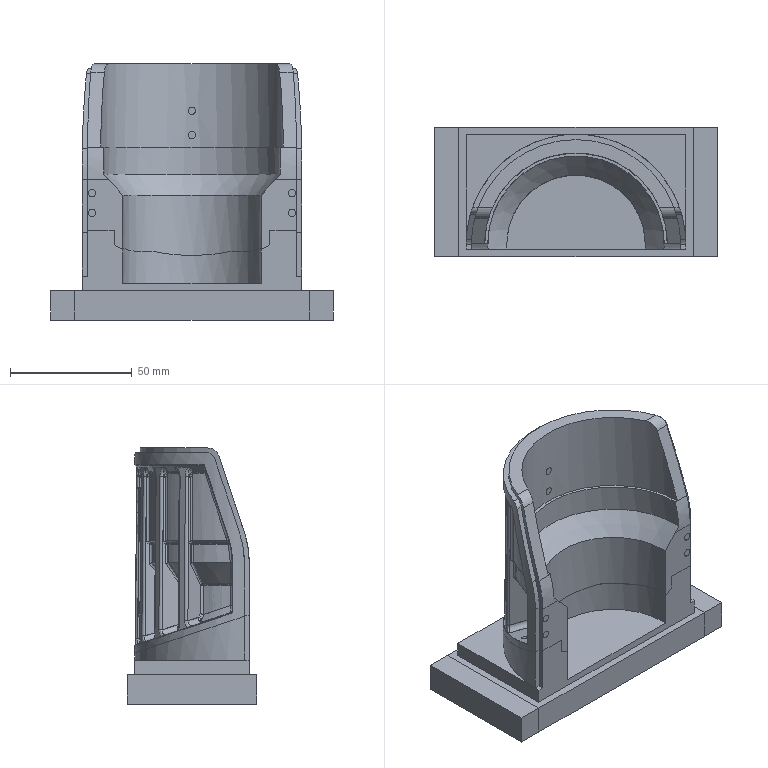CAM job | NX | 3-axis milling, 5-axis milling | part box 116 x 53 x 105 mm
Tools:
number,name,description,diameter,corner_radius,flute_length,length,flutes
16,J-D16,Milling Tool-5 Parameters,16.0,0.0,40.0,80.0,21
18,C-D10,Milling Tool-5 Parameters,10.0,0.0,30.0,45.0,21
14,C-D8,Milling Tool-5 Parameters,8.0,0.0,20.0,35.0,21
12,C-D4,Milling Tool-5 Parameters,4.0,0.0,10.0,25.0,21
6,C-D4R2,Milling Tool-5 Parameters,4.0,2.0,10.0,25.0,21
12,J-D4,Milling Tool-5 Parameters,4.0,0.0,10.0,25.0,21
10,J-D2,Milling Tool-5 Parameters,2.0,0.0,6.0,8.0,21
22,J-D10R0.5,Milling Tool-5 Parameters,10.0,0.5,30.0,55.0,21
21,J-D2R0.2,Milling Tool-5 Parameters,2.0,0.2,6.0,6.0,21
6,J-D4R2,Milling Tool-Ball Mill,4.0,2.0,10.0,25.0,2
8,J-D2R1,Milling Tool-Ball Mill,2.0,1.0,6.0,6.0,2
9,J-D1R0.5,Milling Tool-Ball Mill,1.0,0.5,3.0,3.0,2
7,J-D0.5R0.25,Milling Tool-5 Parameters,0.5,0.25,2.0,2.0,21
Operations:
program,operation,operation_type,tool,method,geometry_group,spindle_rpm,surface_speed,feed_per_tooth,feed_cut,feed_plunge,cut_length_mm,path_length_mm,cut_time_min,machine_time_min
A1,精飞平面,FaceMilling,C-D10,END_MILL_MACRO,WP-1,7000.0,829.0,0.1515,1500.0,100.0,797.45,877.25,0.5316,0.5396
A1,动态开粗,SurfaceContour,C-D10,END_MILL_MACRO,WP-1,7000.0,0.0,0.0,3500.0,100.0,59852.399,81581.703,12.618,14.791
A1,动态开粗_COPY,SurfaceContour,C-D10,END_MILL_MACRO,WP-1,7000.0,0.0,0.0,3500.0,100.0,64037.473,77543.878,13.518,14.868
A1,底壁-跟随,VolumeBased25DMillingOperation,C-D10,METHOD,WP-1,7000.0,87.0,0.2143,500.0,100.0,720.345,878.17,1.441,1.456
A1,底壁-跟随_COPY,VolumeBased25DMillingOperation,C-D10,METHOD,WP-1,7000.0,87.0,0.2143,500.0,100.0,224.0,381.776,0.448,0.4638
A1,剩余铣粗,CavityMilling,C-D10,METHOD,WP-1,7000.0,100.0,0.1178,3500.0,100.0,9658.396,19375.124,2.76,3.731
A1,剩余铣粗_COPY,CavityMilling,C-D10,METHOD,WP-1,7000.0,100.0,0.1178,3500.0,100.0,7296.167,14032.108,2.085,2.758
A1,精爬面,SurfaceContour,C-D10,METHOD,WP-1,7000.0,219.911,0.0102,1500.0,100.0,5400.471,10074.737,3.6,4.068
A2,剩余铣粗_1,CavityMilling,C-D4,METHOD,WP-1,7000.0,100.0,0.1178,3500.0,100.0,3566.135,5871.644,1.019,1.249
A2,剩余铣粗_1_COPY,CavityMilling,C-D4,METHOD,WP-1,7000.0,100.0,0.1178,3500.0,100.0,3352.533,5292.02,0.9579,1.152
A2,剩余铣粗_1_COPY_COPY,CavityMilling,C-D4,METHOD,WP-1,7000.0,100.0,0.1178,3500.0,100.0,3259.975,3977.24,0.9314,1.003
A2,剩余铣粗_1_COPY_COPY_COPY,CavityMilling,C-D4,METHOD,WP-1,7000.0,100.0,0.1178,3500.0,100.0,4154.568,4839.04,1.187,1.256
A2,剩余铣粗_1_COPY_COPY_COPY_COPY,CavityMilling,C-D4,METHOD,WP-1,7000.0,100.0,0.1178,3500.0,100.0,4601.008,5199.555,1.315,1.374
A2,剩余铣粗_1_COPY_COPY_COPY_COPY_COPY,CavityMilling,C-D4,METHOD,WP-1,7000.0,100.0,0.1178,3500.0,100.0,4824.636,5468.098,1.379,1.443
A2,剩余铣粗_1_COPY_COPY_COPY_COPY_COPY_COPY,CavityMilling,C-D4,METHOD,WP-1,7000.0,100.0,0.1178,3500.0,100.0,4042.646,4722.087,1.155,1.223
A2,剩余铣粗_1_COPY_COPY_COPY_COPY_COPY_COPY_COPY,CavityMilling,C-D4,METHOD,WP-1,7000.0,100.0,0.1178,3500.0,100.0,3298.926,4234.6,0.9426,1.036
A2,等高混合,ZLevelMilling,C-D4,METHOD,WP-1,8000.0,122.0,0.0044,2500.0,250.0,1422.571,1699.939,0.5983,0.6261
A2,五轴外形轮廓,SurfaceContour,C-D4,METHOD,WP-1,3500.0,0.0,0.0,600.0,100.0,442.58,1012.272,0.7376,0.7946
A2,五轴外形轮廓_INSTANCE,SurfaceContour,C-D4,METHOD,WP-1,3500.0,0.0,0.0,600.0,100.0,442.58,1012.272,0.7376,0.7946
A2,小孔开粗1,CylinderMilling,C-D4,METHOD,1-A,7000.0,0.0,0.0,600.0,100.0,271.272,447.005,0.4521,0.4697
A2,精大孔-1,PlanarMilling,C-D4,METHOD,1-A,7000.0,188.0,0.0063,200.0,250.0,42.382,208.58,0.2056,0.2223
A3,小孔开粗1_1,CylinderMilling,J-D2,METHOD,1-A,7000.0,0.0,0.0,600.0,100.0,321.786,497.146,0.5363,0.5538
A3,小孔开粗1_1_COPY,CylinderMilling,J-D2,METHOD,1-A,7000.0,0.0,0.0,600.0,100.0,1219.353,1665.353,2.032,2.077
A4,顶面-单刀,SurfaceContour,J-D16,METHOD,WP-1,4000.0,0.0,0.0,500.0,100.0,133.562,139.418,0.2671,0.2677
A4,底壁-跟随_1,VolumeBased25DMillingOperation,J-D16,METHOD,WP-1,4000.0,87.0,0.2143,500.0,100.0,563.041,721.065,1.126,1.142
A4,底壁-跟随_1_COPY,VolumeBased25DMillingOperation,J-D16,METHOD,WP-1,4000.0,87.0,0.2143,500.0,100.0,236.899,394.875,0.4738,0.4896
A4,底壁-跟随_1_COPY_COPY,VolumeBased25DMillingOperation,J-D16,METHOD,WP-1,4000.0,87.0,0.2143,500.0,100.0,150.899,265.899,0.3018,0.3133
A4,底壁-跟随_1_COPY_COPY_COPY,VolumeBased25DMillingOperation,J-D16,METHOD,WP-1,4000.0,87.0,0.2143,500.0,100.0,150.899,265.899,0.3018,0.3133
A5,精外形-1,PlanarMilling,J-D16,METHOD,WP-1,2000.0,100.531,0.0095,400.0,250.0,209.09,534.409,0.5414,0.5739
A5,精外形-1_COPY,PlanarMilling,J-D16,METHOD,WP-1,2000.0,100.531,0.0095,400.0,250.0,208.179,575.005,0.5391,0.5758
A5,精外形-1_COPY_COPY,PlanarMilling,J-D16,METHOD,WP-1,2000.0,100.531,0.0095,400.0,250.0,287.905,514.838,0.738,0.7607
A6,等高混合_1,ZLevelMilling,J-D10R0.5,METHOD,WP-1,8000.0,122.0,0.0044,2500.0,250.0,7195.714,7374.63,2.889,2.907
A7,精爬面_1,SurfaceContour,C-D4R2,METHOD,WP-1,9000.0,0.0,0.0,3500.0,100.0,1893.178,2136.544,0.5409,0.5652
A7,可变轴引导,SurfaceContour,C-D4R2,METHOD,WP-1,9000.0,0.0,0.0,3500.0,250.0,6901.077,6940.344,1.988,1.992
A7,可变轴引导_COPY,SurfaceContour,C-D4R2,METHOD,WP-1,9000.0,0.0,0.0,3500.0,250.0,46895.259,46939.779,13.418,13.422
A8,精爬面_1_COPY,SurfaceContour,J-D4R2,METHOD,WP-1,9000.0,0.0,0.0,3500.0,100.0,4760.29,5004.578,1.36,1.385
A8,可变轴引导_COPY_1,SurfaceContour,J-D4R2,METHOD,WP-1,9000.0,0.0,0.0,3500.0,250.0,17210.697,17250.165,4.934,4.938
A8,精爬面_2,SurfaceContour,J-D4R2,METHOD,1-A,9000.0,0.0,0.0,3500.0,100.0,15374.762,17000.133,4.393,4.555
A8,精爬面_2_COPY,SurfaceContour,J-D4R2,METHOD,1-A,9000.0,0.0,0.0,3500.0,100.0,14600.794,16451.231,4.172,4.357
A8,精爬面_2_COPY_COPY,SurfaceContour,J-D4R2,METHOD,1-A,9000.0,0.0,0.0,3500.0,100.0,13730.005,15511.089,3.923,4.101
A8,精爬面_2_COPY_COPY_COPY,SurfaceContour,J-D4R2,METHOD,1-A,9000.0,0.0,0.0,3500.0,100.0,14590.154,16651.947,4.169,4.375
A8,精爬面_2_COPY_COPY_COPY_COPY,SurfaceContour,J-D4R2,METHOD,1-A,9000.0,0.0,0.0,3500.0,100.0,15019.063,17213.991,4.291,4.511
A8,精爬面_2_COPY_COPY_COPY_COPY_COPY,SurfaceContour,J-D4R2,METHOD,1-A,9000.0,0.0,0.0,3500.0,100.0,15038.602,17141.587,4.297,4.507
A8,精爬面_2_COPY_COPY_COPY_COPY_COPY_COPY,SurfaceContour,J-D4R2,METHOD,1-A,9000.0,0.0,0.0,3500.0,100.0,14575.664,16540.671,4.165,4.361
A8,精爬面_2_COPY_COPY_COPY_COPY_COPY_COPY_COPY,SurfaceContour,J-D4R2,METHOD,1-A,9000.0,0.0,0.0,3500.0,100.0,13832.059,15578.799,3.952,4.127
A9,可变轴引导_COPY_1_COPY_COPY,SurfaceContour,J-D1R0.5,METHOD,1-A,9000.0,0.0,0.0,2500.0,250.0,8473.329,8537.403,3.404,3.41
A9,可变轴引导_COPY_1_COPY_COPY_COPY,SurfaceContour,J-D0.5R0.25,METHOD,1-A,9000.0,0.0,0.0,1500.0,250.0,5434.142,5498.172,3.641,3.647
A10,可变轴引导_COPY_1_COPY,SurfaceContour,J-D2R1,METHOD,1-A,9000.0,0.0,0.0,3500.0,250.0,1642.524,5348.458,0.9096,1.28
A10,精爬面_2_COPY_COPY_COPY_COPY_COPY_COPY_COPY_COPY,SurfaceContour,J-D2R1,METHOD,1-A,9000.0,0.0,0.0,3500.0,100.0,2299.45,2764.825,0.657,0.7035
A10,精爬面_2_COPY_COPY_COPY_COPY_COPY_COPY_COPY_COPY_COPY,SurfaceContour,J-D2R1,METHOD,1-A,9000.0,0.0,0.0,3500.0,100.0,2419.968,2778.237,0.6914,0.7272
A10,精爬面_2_COPY_COPY_COPY_COPY_COPY_COPY_COPY_COPY_COPY_COPY,SurfaceContour,J-D2R1,METHOD,1-A,9000.0,0.0,0.0,3500.0,100.0,2550.904,2916.441,0.7288,0.7654
A10,精爬面_2_COPY_COPY_COPY_COPY_COPY_COPY_COPY_COPY_COPY_COPY_COPY,SurfaceContour,J-D2R1,METHOD,1-A,9000.0,0.0,0.0,3500.0,100.0,2619.79,3131.519,0.7485,0.7997
A10,精爬面_2_COPY_COPY_COPY_COPY_COPY_COPY_COPY_COPY_COPY_COPY_COPY_COPY,SurfaceContour,J-D2R1,METHOD,1-A,9000.0,0.0,0.0,3500.0,100.0,2520.27,2889.356,0.7201,0.757
A10,精爬面_2_COPY_COPY_COPY_COPY_COPY_COPY_COPY_COPY_COPY_COPY_COPY_COPY_COPY,SurfaceContour,J-D2R1,METHOD,1-A,9000.0,0.0,0.0,3500.0,100.0,2490.692,2950.263,0.7116,0.7576
A10,精爬面_2_COPY_COPY_COPY_COPY_COPY_COPY_COPY_COPY_COPY_COPY_COPY_COPY_COPY_COPY,SurfaceContour,J-D2R1,METHOD,1-A,9000.0,0.0,0.0,3500.0,100.0,2399.132,2850.657,0.6855,0.7306
A10,清根顺铣,SurfaceContour,J-D2R1,METHOD,1-A,9000.0,0.0,0.0,2500.0,100.0,5442.728,5814.849,2.177,2.214
A10,清根顺铣_COPY,SurfaceContour,J-D2R1,METHOD,1-A,9000.0,0.0,0.0,2500.0,100.0,5065.634,5409.969,2.026,2.061
A10,清根顺铣_COPY_COPY,SurfaceContour,J-D2R1,METHOD,1-A,9000.0,0.0,0.0,2500.0,100.0,5242.358,5516.055,2.097,2.124
A10,清根顺铣_COPY_COPY_COPY,SurfaceContour,J-D2R1,METHOD,1-A,9000.0,0.0,0.0,2500.0,100.0,5063.953,5345.31,2.026,2.054
A10,清根顺铣_COPY_COPY_COPY_COPY,SurfaceContour,J-D2R1,METHOD,1-A,9000.0,0.0,0.0,2500.0,100.0,5132.172,5427.779,2.053,2.082
A10,清根顺铣_COPY_COPY_COPY_COPY_COPY,SurfaceContour,J-D2R1,METHOD,1-A,9000.0,0.0,0.0,2500.0,100.0,4797.782,5093.276,1.919,1.949
A10,清根顺铣_COPY_COPY_COPY_COPY_COPY_COPY,SurfaceContour,J-D2R1,METHOD,1-A,9000.0,0.0,0.0,2500.0,100.0,5087.474,5399.538,2.035,2.066
A10,清根顺铣_COPY_COPY_COPY_COPY_COPY_COPY_COPY,SurfaceContour,J-D2R1,METHOD,1-A,9000.0,0.0,0.0,2500.0,100.0,5239.47,5511.892,2.096,2.123
A10,三轴去毛刺,TpMultiAxisDeburring,J-D2R1,METHOD,1-A,9000.0,0.0,0.0,1000.0,90.0,16.468,158.458,0.0168,0.0168
A10,三轴去毛刺_COPY,TpMultiAxisDeburring,J-D2R1,METHOD,1-A,9000.0,0.0,0.0,1000.0,90.0,49.191,674.186,0.0501,0.0501
A10,五轴去毛刺,TpMultiAxisDeburring,J-D2R1,METHOD,1-A,9000.0,0.0,0.0,1000.0,90.0,254.038,266.376,0.2542,0.2542
A11,等高混合_2,ZLevelMilling,J-D2R0.2,METHOD,1-A,8000.0,122.0,0.0044,1500.0,250.0,1226.637,1385.879,0.9298,0.9457
A11,等高混合_2_COPY,ZLevelMilling,J-D2R0.2,METHOD,1-A,8000.0,122.0,0.0044,1500.0,250.0,396.512,602.2,0.3519,0.3725
B1,动态开粗_1,SurfaceContour,C-D8,METHOD,2-A,10000.0,251.327,0.0119,2500.0,100.0,30341.604,30382.204,7.765,7.769
B1,型腔开粗1,CavityMilling,C-D8,METHOD,2-A,10000.0,251.327,0.0119,2500.0,100.0,84879.924,87286.557,33.952,34.193
B1,等高混合_3,ZLevelMilling,C-D8,METHOD,WP-2,8000.0,122.0,0.0044,2500.0,250.0,227.727,589.938,0.1114,0.1477
B1,底壁-跟随_2,VolumeBased25DMillingOperation,C-D8,METHOD,WP-2,7000.0,87.0,0.2143,500.0,100.0,757.282,908.649,1.515,1.53
B1,精爬面_3,SurfaceContour,C-D4R2,METHOD,WP-2,9000.0,0.0,0.0,3500.0,100.0,1127.2,1473.819,0.3221,0.3567
B2,底壁-往复,VolumeBased25DMillingOperation,J-D4,METHOD,WP-2,7000.0,87.0,0.2143,500.0,100.0,1199.856,1351.324,2.4,2.415
B3,等高混合_4,ZLevelMilling,J-D2R0.2,METHOD,WP-2,8000.0,122.0,0.0044,2000.0,250.0,3410.577,4006.346,1.745,1.804
B3,小孔开粗1_2,CylinderMilling,J-D2R0.2,METHOD,WP-2,8000.0,0.0,0.0,600.0,100.0,726.032,1468.027,1.21,1.284
B4,精爬面_3_COPY,SurfaceContour,J-D2R1,METHOD,WP-2,9000.0,0.0,0.0,3500.0,100.0,3440.559,3656.624,0.983,1.005